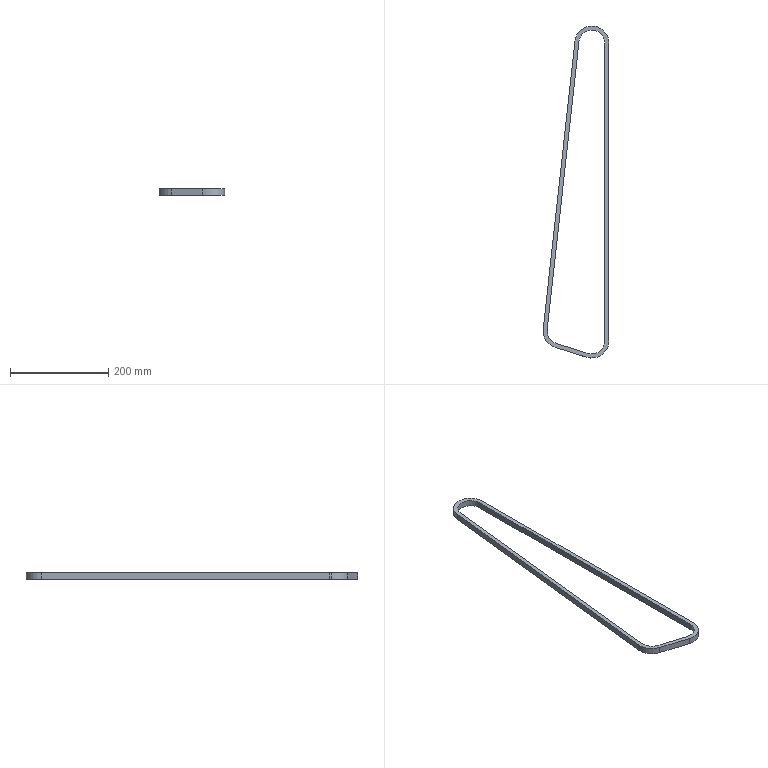Part | STEP file | Belt 1-2^Lifting mechanism | 1 solid | 16 faces | box 133.82 x 674.32 x 12.8 mm | volume 154708 mm3 | cylinder 8 | plane 8 | commonest cylinder face diameters 52.68 x4 69.32 x4
STEP:
#1=CARTESIAN_POINT('',(0.,0.,0.));
#2=DIRECTION('',(0.,0.,1.));
#3=DIRECTION('',(1.,0.,0.));
#4=AXIS2_PLACEMENT_3D('',#1,#2,#3);
#5=CARTESIAN_POINT('',(-90.681,22.887,6.4));
#6=VERTEX_POINT('',#5);
#7=CARTESIAN_POINT('',(-90.681,22.887,-6.4));
#8=VERTEX_POINT('',#7);
#9=CARTESIAN_POINT('',(-90.681,22.887,6.4));
#10=DIRECTION('',(0.,0.,-1.));
#11=VECTOR('',#10,1.);
#12=LINE('',#9,#11);
#13=CARTESIAN_POINT('',(-64.5,20.,6.4));
#14=DIRECTION('',(0.,0.,-1.));
#15=DIRECTION('',(-1.,0.,0.));
#16=AXIS2_PLACEMENT_3D('',#13,#14,#15);
#17=CYLINDRICAL_SURFACE('',#16,26.34);
#18=CARTESIAN_POINT('',(0.1098,0.));
#19=DIRECTION('',(0.,1.));
#20=VECTOR('',#19,1.);
#21=LINE('',#18,#20);
#22=(GEOMETRIC_REPRESENTATION_CONTEXT(2)PARAMETRIC_REPRESENTATION_CONTEXT()REPRESENTATION_CONTEXT('',''));
#23=DEFINITIONAL_REPRESENTATION('',(#21),#22);
#24=PCURVE('',#17,#23);
#25=CARTESIAN_POINT('',(-92.085,10.153,6.4));
#26=DIRECTION('',(0.994,-0.1096,0.));
#27=DIRECTION('',(0.1096,0.994,0.));
#28=AXIS2_PLACEMENT_3D('',#25,#26,#27);
#29=PLANE('',#28);
#30=CARTESIAN_POINT('',(12.811,0.));
#31=DIRECTION('',(0.,-1.));
#32=VECTOR('',#31,1.);
#33=LINE('',#30,#32);
#34=(GEOMETRIC_REPRESENTATION_CONTEXT(2)PARAMETRIC_REPRESENTATION_CONTEXT()REPRESENTATION_CONTEXT('',''));
#35=DEFINITIONAL_REPRESENTATION('',(#33),#34);
#36=PCURVE('',#29,#35);
#37=SURFACE_CURVE('',#12,(#24,#36),.PCURVE_S1.);
#38=EDGE_CURVE('',#6,#8,#37,.T.);
#39=ORIENTED_EDGE('',*,*,#38,.T.);
#40=CARTESIAN_POINT('',(-90.84,20.,-6.4));
#41=VERTEX_POINT('',#40);
#42=CARTESIAN_POINT('',(-64.5,20.,-6.4));
#43=DIRECTION('',(0.,0.,1.));
#44=DIRECTION('',(-1.,0.,0.));
#45=AXIS2_PLACEMENT_3D('',#42,#43,#44);
#46=CIRCLE('',#45,26.34);
#47=CARTESIAN_POINT('',(6.283,12.8));
#48=DIRECTION('',(-1.,0.));
#49=VECTOR('',#48,1.);
#50=LINE('',#47,#49);
#51=(GEOMETRIC_REPRESENTATION_CONTEXT(2)PARAMETRIC_REPRESENTATION_CONTEXT()REPRESENTATION_CONTEXT('',''));
#52=DEFINITIONAL_REPRESENTATION('',(#50),#51);
#53=PCURVE('',#17,#52);
#54=CARTESIAN_POINT('',(0.,0.,-6.4));
#55=DIRECTION('',(0.,0.,-1.));
#56=DIRECTION('',(-1.,0.,0.));
#57=AXIS2_PLACEMENT_3D('',#54,#55,#56);
#58=PLANE('',#57);
#59=CARTESIAN_POINT('',(90.84,20.));
#60=CARTESIAN_POINT('',(90.84,-25.622));
#61=CARTESIAN_POINT('',(51.33,-2.811));
#62=CARTESIAN_POINT('',(11.82,20.));
#63=CARTESIAN_POINT('',(51.33,42.811));
#64=CARTESIAN_POINT('',(90.84,65.622));
#65=CARTESIAN_POINT('',(90.84,20.));
#66=(BOUNDED_CURVE()B_SPLINE_CURVE(2,(#59,#60,#61,#62,#63,#64,#65),.UNSPECIFIED.,.T.,.F.)B_SPLINE_CURVE_WITH_KNOTS((1,2,2,2,2,1),(-2.094,0.,2.094,4.189,6.283,8.378),.UNSPECIFIED.)CURVE()GEOMETRIC_REPRESENTATION_ITEM()RATIONAL_B_SPLINE_CURVE((1.,0.5,1.,0.5,1.,0.5,1.))REPRESENTATION_ITEM(''));
#67=(GEOMETRIC_REPRESENTATION_CONTEXT(2)PARAMETRIC_REPRESENTATION_CONTEXT()REPRESENTATION_CONTEXT('',''));
#68=DEFINITIONAL_REPRESENTATION('',(#66),#67);
#69=PCURVE('',#58,#68);
#70=SURFACE_CURVE('',#46,(#53,#69),.PCURVE_S1.);
#71=EDGE_CURVE('',#8,#41,#70,.T.);
#72=ORIENTED_EDGE('',*,*,#71,.T.);
#73=CARTESIAN_POINT('',(-90.84,20.,6.4));
#74=VERTEX_POINT('',#73);
#75=CARTESIAN_POINT('',(-90.84,20.,6.4));
#76=DIRECTION('',(0.,0.,-1.));
#77=VECTOR('',#76,1.);
#78=LINE('',#75,#77);
#79=CARTESIAN_POINT('',(0.,0.));
#80=DIRECTION('',(0.,1.));
#81=VECTOR('',#80,1.);
#82=LINE('',#79,#81);
#83=(GEOMETRIC_REPRESENTATION_CONTEXT(2)PARAMETRIC_REPRESENTATION_CONTEXT()REPRESENTATION_CONTEXT('',''));
#84=DEFINITIONAL_REPRESENTATION('',(#82),#83);
#85=PCURVE('',#17,#84);
#86=CARTESIAN_POINT('',(-64.5,20.,6.4));
#87=DIRECTION('',(0.,0.,-1.));
#88=DIRECTION('',(-1.,0.,0.));
#89=AXIS2_PLACEMENT_3D('',#86,#87,#88);
#90=CYLINDRICAL_SURFACE('',#89,26.34);
#91=CARTESIAN_POINT('',(6.283,0.));
#92=DIRECTION('',(0.,1.));
#93=VECTOR('',#92,1.);
#94=LINE('',#91,#93);
#95=(GEOMETRIC_REPRESENTATION_CONTEXT(2)PARAMETRIC_REPRESENTATION_CONTEXT()REPRESENTATION_CONTEXT('',''));
#96=DEFINITIONAL_REPRESENTATION('',(#94),#95);
#97=PCURVE('',#90,#96);
#98=SURFACE_CURVE('',#78,(#85,#97),.PCURVE_S1.);
#99=EDGE_CURVE('',#74,#41,#98,.T.);
#100=ORIENTED_EDGE('',*,*,#99,.F.);
#101=CARTESIAN_POINT('',(-64.5,20.,6.4));
#102=DIRECTION('',(0.,0.,1.));
#103=DIRECTION('',(-1.,0.,0.));
#104=AXIS2_PLACEMENT_3D('',#101,#102,#103);
#105=CIRCLE('',#104,26.34);
#106=CARTESIAN_POINT('',(6.283,0.));
#107=DIRECTION('',(-1.,0.));
#108=VECTOR('',#107,1.);
#109=LINE('',#106,#108);
#110=(GEOMETRIC_REPRESENTATION_CONTEXT(2)PARAMETRIC_REPRESENTATION_CONTEXT()REPRESENTATION_CONTEXT('',''));
#111=DEFINITIONAL_REPRESENTATION('',(#109),#110);
#112=PCURVE('',#17,#111);
#113=CARTESIAN_POINT('',(0.,0.,6.4));
#114=DIRECTION('',(0.,0.,-1.));
#115=DIRECTION('',(-1.,0.,0.));
#116=AXIS2_PLACEMENT_3D('',#113,#114,#115);
#117=PLANE('',#116);
#118=CARTESIAN_POINT('',(90.84,20.));
#119=CARTESIAN_POINT('',(90.84,-25.622));
#120=CARTESIAN_POINT('',(51.33,-2.811));
#121=CARTESIAN_POINT('',(11.82,20.));
#122=CARTESIAN_POINT('',(51.33,42.811));
#123=CARTESIAN_POINT('',(90.84,65.622));
#124=CARTESIAN_POINT('',(90.84,20.));
#125=(BOUNDED_CURVE()B_SPLINE_CURVE(2,(#118,#119,#120,#121,#122,#123,#124),.UNSPECIFIED.,.T.,.F.)B_SPLINE_CURVE_WITH_KNOTS((1,2,2,2,2,1),(-2.094,0.,2.094,4.189,6.283,8.378),.UNSPECIFIED.)CURVE()GEOMETRIC_REPRESENTATION_ITEM()RATIONAL_B_SPLINE_CURVE((1.,0.5,1.,0.5,1.,0.5,1.))REPRESENTATION_ITEM(''));
#126=(GEOMETRIC_REPRESENTATION_CONTEXT(2)PARAMETRIC_REPRESENTATION_CONTEXT()REPRESENTATION_CONTEXT('',''));
#127=DEFINITIONAL_REPRESENTATION('',(#125),#126);
#128=PCURVE('',#117,#127);
#129=SURFACE_CURVE('',#105,(#112,#128),.PCURVE_S1.);
#130=EDGE_CURVE('',#6,#74,#129,.T.);
#131=ORIENTED_EDGE('',*,*,#130,.F.);
#132=EDGE_LOOP('',(#39,#72,#100,#131));
#133=FACE_BOUND('',#132,.F.);
#134=ADVANCED_FACE('',(#133),#17,.F.);
#135=CARTESIAN_POINT('',(-99.16,20.,6.4));
#136=VERTEX_POINT('',#135);
#137=CARTESIAN_POINT('',(-74.765,-13.105,6.4));
#138=VERTEX_POINT('',#137);
#139=CARTESIAN_POINT('',(-64.5,20.,6.4));
#140=DIRECTION('',(0.,0.,1.));
#141=DIRECTION('',(-1.,0.,0.));
#142=AXIS2_PLACEMENT_3D('',#139,#140,#141);
#143=CIRCLE('',#142,34.66);
#144=CARTESIAN_POINT('',(-64.5,20.,6.4));
#145=DIRECTION('',(0.,0.,-1.));
#146=DIRECTION('',(-1.,0.,0.));
#147=AXIS2_PLACEMENT_3D('',#144,#145,#146);
#148=CYLINDRICAL_SURFACE('',#147,34.66);
#149=CARTESIAN_POINT('',(6.283,0.));
#150=DIRECTION('',(-1.,0.));
#151=VECTOR('',#150,1.);
#152=LINE('',#149,#151);
#153=(GEOMETRIC_REPRESENTATION_CONTEXT(2)PARAMETRIC_REPRESENTATION_CONTEXT()REPRESENTATION_CONTEXT('',''));
#154=DEFINITIONAL_REPRESENTATION('',(#152),#153);
#155=PCURVE('',#148,#154);
#156=CARTESIAN_POINT('',(99.16,20.));
#157=CARTESIAN_POINT('',(99.16,-40.033));
#158=CARTESIAN_POINT('',(47.17,-10.016));
#159=CARTESIAN_POINT('',(-4.82,20.));
#160=CARTESIAN_POINT('',(47.17,50.016));
#161=CARTESIAN_POINT('',(99.16,80.033));
#162=CARTESIAN_POINT('',(99.16,20.));
#163=(BOUNDED_CURVE()B_SPLINE_CURVE(2,(#156,#157,#158,#159,#160,#161,#162),.UNSPECIFIED.,.T.,.F.)B_SPLINE_CURVE_WITH_KNOTS((1,2,2,2,2,1),(-2.094,0.,2.094,4.189,6.283,8.378),.UNSPECIFIED.)CURVE()GEOMETRIC_REPRESENTATION_ITEM()RATIONAL_B_SPLINE_CURVE((1.,0.5,1.,0.5,1.,0.5,1.))REPRESENTATION_ITEM(''));
#164=(GEOMETRIC_REPRESENTATION_CONTEXT(2)PARAMETRIC_REPRESENTATION_CONTEXT()REPRESENTATION_CONTEXT('',''));
#165=DEFINITIONAL_REPRESENTATION('',(#163),#164);
#166=PCURVE('',#117,#165);
#167=SURFACE_CURVE('',#143,(#155,#166),.PCURVE_S1.);
#168=EDGE_CURVE('',#136,#138,#167,.T.);
#169=ORIENTED_EDGE('',*,*,#168,.F.);
#170=CARTESIAN_POINT('',(-99.16,20.,-6.4));
#171=VERTEX_POINT('',#170);
#172=CARTESIAN_POINT('',(-99.16,20.,6.4));
#173=DIRECTION('',(0.,0.,-1.));
#174=VECTOR('',#173,1.);
#175=LINE('',#172,#174);
#176=CARTESIAN_POINT('',(6.283,0.));
#177=DIRECTION('',(0.,1.));
#178=VECTOR('',#177,1.);
#179=LINE('',#176,#178);
#180=(GEOMETRIC_REPRESENTATION_CONTEXT(2)PARAMETRIC_REPRESENTATION_CONTEXT()REPRESENTATION_CONTEXT('',''));
#181=DEFINITIONAL_REPRESENTATION('',(#179),#180);
#182=PCURVE('',#148,#181);
#183=CARTESIAN_POINT('',(-64.5,20.,6.4));
#184=DIRECTION('',(0.,0.,-1.));
#185=DIRECTION('',(-1.,0.,0.));
#186=AXIS2_PLACEMENT_3D('',#183,#184,#185);
#187=CYLINDRICAL_SURFACE('',#186,34.66);
#188=CARTESIAN_POINT('',(0.,0.));
#189=DIRECTION('',(0.,1.));
#190=VECTOR('',#189,1.);
#191=LINE('',#188,#190);
#192=(GEOMETRIC_REPRESENTATION_CONTEXT(2)PARAMETRIC_REPRESENTATION_CONTEXT()REPRESENTATION_CONTEXT('',''));
#193=DEFINITIONAL_REPRESENTATION('',(#191),#192);
#194=PCURVE('',#187,#193);
#195=SURFACE_CURVE('',#175,(#182,#194),.PCURVE_S1.);
#196=EDGE_CURVE('',#136,#171,#195,.T.);
#197=ORIENTED_EDGE('',*,*,#196,.T.);
#198=CARTESIAN_POINT('',(-74.765,-13.105,-6.4));
#199=VERTEX_POINT('',#198);
#200=CARTESIAN_POINT('',(-64.5,20.,-6.4));
#201=DIRECTION('',(0.,0.,1.));
#202=DIRECTION('',(-1.,0.,0.));
#203=AXIS2_PLACEMENT_3D('',#200,#201,#202);
#204=CIRCLE('',#203,34.66);
#205=CARTESIAN_POINT('',(6.283,12.8));
#206=DIRECTION('',(-1.,0.));
#207=VECTOR('',#206,1.);
#208=LINE('',#205,#207);
#209=(GEOMETRIC_REPRESENTATION_CONTEXT(2)PARAMETRIC_REPRESENTATION_CONTEXT()REPRESENTATION_CONTEXT('',''));
#210=DEFINITIONAL_REPRESENTATION('',(#208),#209);
#211=PCURVE('',#148,#210);
#212=CARTESIAN_POINT('',(99.16,20.));
#213=CARTESIAN_POINT('',(99.16,-40.033));
#214=CARTESIAN_POINT('',(47.17,-10.016));
#215=CARTESIAN_POINT('',(-4.82,20.));
#216=CARTESIAN_POINT('',(47.17,50.016));
#217=CARTESIAN_POINT('',(99.16,80.033));
#218=CARTESIAN_POINT('',(99.16,20.));
#219=(BOUNDED_CURVE()B_SPLINE_CURVE(2,(#212,#213,#214,#215,#216,#217,#218),.UNSPECIFIED.,.T.,.F.)B_SPLINE_CURVE_WITH_KNOTS((1,2,2,2,2,1),(-2.094,0.,2.094,4.189,6.283,8.378),.UNSPECIFIED.)CURVE()GEOMETRIC_REPRESENTATION_ITEM()RATIONAL_B_SPLINE_CURVE((1.,0.5,1.,0.5,1.,0.5,1.))REPRESENTATION_ITEM(''));
#220=(GEOMETRIC_REPRESENTATION_CONTEXT(2)PARAMETRIC_REPRESENTATION_CONTEXT()REPRESENTATION_CONTEXT('',''));
#221=DEFINITIONAL_REPRESENTATION('',(#219),#220);
#222=PCURVE('',#58,#221);
#223=SURFACE_CURVE('',#204,(#211,#222),.PCURVE_S1.);
#224=EDGE_CURVE('',#171,#199,#223,.T.);
#225=ORIENTED_EDGE('',*,*,#224,.T.);
#226=CARTESIAN_POINT('',(-74.765,-13.105,6.4));
#227=DIRECTION('',(0.,0.,-1.));
#228=VECTOR('',#227,1.);
#229=LINE('',#226,#228);
#230=CARTESIAN_POINT('',(5.013,0.));
#231=DIRECTION('',(0.,1.));
#232=VECTOR('',#231,1.);
#233=LINE('',#230,#232);
#234=(GEOMETRIC_REPRESENTATION_CONTEXT(2)PARAMETRIC_REPRESENTATION_CONTEXT()REPRESENTATION_CONTEXT('',''));
#235=DEFINITIONAL_REPRESENTATION('',(#233),#234);
#236=PCURVE('',#148,#235);
#237=CARTESIAN_POINT('',(-10.265,-33.105,6.4));
#238=DIRECTION('',(0.2962,0.9551,0.));
#239=DIRECTION('',(-0.9551,0.2962,0.));
#240=AXIS2_PLACEMENT_3D('',#237,#238,#239);
#241=PLANE('',#240);
#242=CARTESIAN_POINT('',(67.53,0.));
#243=DIRECTION('',(0.,-1.));
#244=VECTOR('',#243,1.);
#245=LINE('',#242,#244);
#246=(GEOMETRIC_REPRESENTATION_CONTEXT(2)PARAMETRIC_REPRESENTATION_CONTEXT()REPRESENTATION_CONTEXT('',''));
#247=DEFINITIONAL_REPRESENTATION('',(#245),#246);
#248=PCURVE('',#241,#247);
#249=SURFACE_CURVE('',#229,(#236,#248),.PCURVE_S1.);
#250=EDGE_CURVE('',#138,#199,#249,.T.);
#251=ORIENTED_EDGE('',*,*,#250,.F.);
#252=EDGE_LOOP('',(#169,#197,#225,#251));
#253=FACE_BOUND('',#252,.T.);
#254=ADVANCED_FACE('',(#253),#148,.T.);
#255=CARTESIAN_POINT('',(-10.265,-33.105,6.4));
#256=VERTEX_POINT('',#255);
#257=CARTESIAN_POINT('',(34.66,0.,6.4));
#258=VERTEX_POINT('',#257);
#259=CARTESIAN_POINT('',(0.,0.,6.4));
#260=DIRECTION('',(0.,0.,1.));
#261=DIRECTION('',(-1.,0.,0.));
#262=AXIS2_PLACEMENT_3D('',#259,#260,#261);
#263=CIRCLE('',#262,34.66);
#264=CARTESIAN_POINT('',(34.66,0.));
#265=CARTESIAN_POINT('',(34.66,-60.033));
#266=CARTESIAN_POINT('',(-17.33,-30.016));
#267=CARTESIAN_POINT('',(-69.32,0.));
#268=CARTESIAN_POINT('',(-17.33,30.016));
#269=CARTESIAN_POINT('',(34.66,60.033));
#270=CARTESIAN_POINT('',(34.66,0.));
#271=(BOUNDED_CURVE()B_SPLINE_CURVE(2,(#264,#265,#266,#267,#268,#269,#270),.UNSPECIFIED.,.T.,.F.)B_SPLINE_CURVE_WITH_KNOTS((1,2,2,2,2,1),(-2.094,0.,2.094,4.189,6.283,8.378),.UNSPECIFIED.)CURVE()GEOMETRIC_REPRESENTATION_ITEM()RATIONAL_B_SPLINE_CURVE((1.,0.5,1.,0.5,1.,0.5,1.))REPRESENTATION_ITEM(''));
#272=(GEOMETRIC_REPRESENTATION_CONTEXT(2)PARAMETRIC_REPRESENTATION_CONTEXT()REPRESENTATION_CONTEXT('',''));
#273=DEFINITIONAL_REPRESENTATION('',(#271),#272);
#274=PCURVE('',#117,#273);
#275=CARTESIAN_POINT('',(0.,0.,6.4));
#276=DIRECTION('',(0.,0.,-1.));
#277=DIRECTION('',(-1.,0.,0.));
#278=AXIS2_PLACEMENT_3D('',#275,#276,#277);
#279=CYLINDRICAL_SURFACE('',#278,34.66);
#280=CARTESIAN_POINT('',(6.283,0.));
#281=DIRECTION('',(-1.,0.));
#282=VECTOR('',#281,1.);
#283=LINE('',#280,#282);
#284=(GEOMETRIC_REPRESENTATION_CONTEXT(2)PARAMETRIC_REPRESENTATION_CONTEXT()REPRESENTATION_CONTEXT('',''));
#285=DEFINITIONAL_REPRESENTATION('',(#283),#284);
#286=PCURVE('',#279,#285);
#287=SURFACE_CURVE('',#263,(#274,#286),.PCURVE_S1.);
#288=EDGE_CURVE('',#256,#258,#287,.T.);
#289=ORIENTED_EDGE('',*,*,#288,.T.);
#290=CARTESIAN_POINT('',(34.66,605.,6.4));
#291=VERTEX_POINT('',#290);
#292=CARTESIAN_POINT('',(34.66,0.,6.4));
#293=DIRECTION('',(0.,1.,0.));
#294=VECTOR('',#293,1.);
#295=LINE('',#292,#294);
#296=CARTESIAN_POINT('',(-34.66,0.));
#297=DIRECTION('',(0.,1.));
#298=VECTOR('',#297,1.);
#299=LINE('',#296,#298);
#300=(GEOMETRIC_REPRESENTATION_CONTEXT(2)PARAMETRIC_REPRESENTATION_CONTEXT()REPRESENTATION_CONTEXT('',''));
#301=DEFINITIONAL_REPRESENTATION('',(#299),#300);
#302=PCURVE('',#117,#301);
#303=CARTESIAN_POINT('',(34.66,0.,6.4));
#304=DIRECTION('',(-1.,0.,0.));
#305=DIRECTION('',(0.,-1.,0.));
#306=AXIS2_PLACEMENT_3D('',#303,#304,#305);
#307=PLANE('',#306);
#308=CARTESIAN_POINT('',(0.,0.));
#309=DIRECTION('',(-1.,0.));
#310=VECTOR('',#309,1.);
#311=LINE('',#308,#310);
#312=(GEOMETRIC_REPRESENTATION_CONTEXT(2)PARAMETRIC_REPRESENTATION_CONTEXT()REPRESENTATION_CONTEXT('',''));
#313=DEFINITIONAL_REPRESENTATION('',(#311),#312);
#314=PCURVE('',#307,#313);
#315=SURFACE_CURVE('',#295,(#302,#314),.PCURVE_S1.);
#316=EDGE_CURVE('',#258,#291,#315,.T.);
#317=ORIENTED_EDGE('',*,*,#316,.T.);
#318=CARTESIAN_POINT('',(-34.451,608.798,6.4));
#319=VERTEX_POINT('',#318);
#320=CARTESIAN_POINT('',(0.,605.,6.4));
#321=DIRECTION('',(0.,0.,1.));
#322=DIRECTION('',(-1.,0.,0.));
#323=AXIS2_PLACEMENT_3D('',#320,#321,#322);
#324=CIRCLE('',#323,34.66);
#325=CARTESIAN_POINT('',(34.66,605.));
#326=CARTESIAN_POINT('',(34.66,544.967));
#327=CARTESIAN_POINT('',(-17.33,574.984));
#328=CARTESIAN_POINT('',(-69.32,605.));
#329=CARTESIAN_POINT('',(-17.33,635.016));
#330=CARTESIAN_POINT('',(34.66,665.033));
#331=CARTESIAN_POINT('',(34.66,605.));
#332=(BOUNDED_CURVE()B_SPLINE_CURVE(2,(#325,#326,#327,#328,#329,#330,#331),.UNSPECIFIED.,.T.,.F.)B_SPLINE_CURVE_WITH_KNOTS((1,2,2,2,2,1),(-2.094,0.,2.094,4.189,6.283,8.378),.UNSPECIFIED.)CURVE()GEOMETRIC_REPRESENTATION_ITEM()RATIONAL_B_SPLINE_CURVE((1.,0.5,1.,0.5,1.,0.5,1.))REPRESENTATION_ITEM(''));
#333=(GEOMETRIC_REPRESENTATION_CONTEXT(2)PARAMETRIC_REPRESENTATION_CONTEXT()REPRESENTATION_CONTEXT('',''));
#334=DEFINITIONAL_REPRESENTATION('',(#332),#333);
#335=PCURVE('',#117,#334);
#336=CARTESIAN_POINT('',(0.,605.,6.4));
#337=DIRECTION('',(0.,0.,-1.));
#338=DIRECTION('',(-1.,0.,0.));
#339=AXIS2_PLACEMENT_3D('',#336,#337,#338);
#340=CYLINDRICAL_SURFACE('',#339,34.66);
#341=CARTESIAN_POINT('',(6.283,0.));
#342=DIRECTION('',(-1.,0.));
#343=VECTOR('',#342,1.);
#344=LINE('',#341,#343);
#345=(GEOMETRIC_REPRESENTATION_CONTEXT(2)PARAMETRIC_REPRESENTATION_CONTEXT()REPRESENTATION_CONTEXT('',''));
#346=DEFINITIONAL_REPRESENTATION('',(#344),#345);
#347=PCURVE('',#340,#346);
#348=SURFACE_CURVE('',#324,(#335,#347),.PCURVE_S1.);
#349=EDGE_CURVE('',#291,#319,#348,.T.);
#350=ORIENTED_EDGE('',*,*,#349,.T.);
#351=CARTESIAN_POINT('',(-98.951,23.798,6.4));
#352=VERTEX_POINT('',#351);
#353=CARTESIAN_POINT('',(-100.355,11.065,6.4));
#354=DIRECTION('',(-0.1096,-0.994,0.));
#355=VECTOR('',#354,1.);
#356=LINE('',#353,#355);
#357=CARTESIAN_POINT('',(100.355,11.065));
#358=DIRECTION('',(0.1096,-0.994));
#359=VECTOR('',#358,1.);
#360=LINE('',#357,#359);
#361=(GEOMETRIC_REPRESENTATION_CONTEXT(2)PARAMETRIC_REPRESENTATION_CONTEXT()REPRESENTATION_CONTEXT('',''));
#362=DEFINITIONAL_REPRESENTATION('',(#360),#361);
#363=PCURVE('',#117,#362);
#364=CARTESIAN_POINT('',(-100.355,11.065,6.4));
#365=DIRECTION('',(0.994,-0.1096,0.));
#366=DIRECTION('',(0.1096,0.994,0.));
#367=AXIS2_PLACEMENT_3D('',#364,#365,#366);
#368=PLANE('',#367);
#369=CARTESIAN_POINT('',(0.,0.));
#370=DIRECTION('',(-1.,0.));
#371=VECTOR('',#370,1.);
#372=LINE('',#369,#371);
#373=(GEOMETRIC_REPRESENTATION_CONTEXT(2)PARAMETRIC_REPRESENTATION_CONTEXT()REPRESENTATION_CONTEXT('',''));
#374=DEFINITIONAL_REPRESENTATION('',(#372),#373);
#375=PCURVE('',#368,#374);
#376=SURFACE_CURVE('',#356,(#363,#375),.PCURVE_S1.);
#377=EDGE_CURVE('',#319,#352,#376,.T.);
#378=ORIENTED_EDGE('',*,*,#377,.T.);
#379=CARTESIAN_POINT('',(-64.5,20.,6.4));
#380=DIRECTION('',(0.,0.,1.));
#381=DIRECTION('',(-1.,0.,0.));
#382=AXIS2_PLACEMENT_3D('',#379,#380,#381);
#383=CIRCLE('',#382,34.66);
#384=CARTESIAN_POINT('',(99.16,20.));
#385=CARTESIAN_POINT('',(99.16,-40.033));
#386=CARTESIAN_POINT('',(47.17,-10.016));
#387=CARTESIAN_POINT('',(-4.82,20.));
#388=CARTESIAN_POINT('',(47.17,50.016));
#389=CARTESIAN_POINT('',(99.16,80.033));
#390=CARTESIAN_POINT('',(99.16,20.));
#391=(BOUNDED_CURVE()B_SPLINE_CURVE(2,(#384,#385,#386,#387,#388,#389,#390),.UNSPECIFIED.,.T.,.F.)B_SPLINE_CURVE_WITH_KNOTS((1,2,2,2,2,1),(-2.094,0.,2.094,4.189,6.283,8.378),.UNSPECIFIED.)CURVE()GEOMETRIC_REPRESENTATION_ITEM()RATIONAL_B_SPLINE_CURVE((1.,0.5,1.,0.5,1.,0.5,1.))REPRESENTATION_ITEM(''));
#392=(GEOMETRIC_REPRESENTATION_CONTEXT(2)PARAMETRIC_REPRESENTATION_CONTEXT()REPRESENTATION_CONTEXT('',''));
#393=DEFINITIONAL_REPRESENTATION('',(#391),#392);
#394=PCURVE('',#117,#393);
#395=CARTESIAN_POINT('',(6.283,0.));
#396=DIRECTION('',(-1.,0.));
#397=VECTOR('',#396,1.);
#398=LINE('',#395,#397);
#399=(GEOMETRIC_REPRESENTATION_CONTEXT(2)PARAMETRIC_REPRESENTATION_CONTEXT()REPRESENTATION_CONTEXT('',''));
#400=DEFINITIONAL_REPRESENTATION('',(#398),#399);
#401=PCURVE('',#187,#400);
#402=SURFACE_CURVE('',#383,(#394,#401),.PCURVE_S1.);
#403=EDGE_CURVE('',#352,#136,#402,.T.);
#404=ORIENTED_EDGE('',*,*,#403,.T.);
#405=ORIENTED_EDGE('',*,*,#168,.T.);
#406=CARTESIAN_POINT('',(-10.265,-33.105,6.4));
#407=DIRECTION('',(0.9551,-0.2962,0.));
#408=VECTOR('',#407,1.);
#409=LINE('',#406,#408);
#410=CARTESIAN_POINT('',(10.265,-33.105));
#411=DIRECTION('',(-0.9551,-0.2962));
#412=VECTOR('',#411,1.);
#413=LINE('',#410,#412);
#414=(GEOMETRIC_REPRESENTATION_CONTEXT(2)PARAMETRIC_REPRESENTATION_CONTEXT()REPRESENTATION_CONTEXT('',''));
#415=DEFINITIONAL_REPRESENTATION('',(#413),#414);
#416=PCURVE('',#117,#415);
#417=CARTESIAN_POINT('',(0.,0.));
#418=DIRECTION('',(-1.,0.));
#419=VECTOR('',#418,1.);
#420=LINE('',#417,#419);
#421=(GEOMETRIC_REPRESENTATION_CONTEXT(2)PARAMETRIC_REPRESENTATION_CONTEXT()REPRESENTATION_CONTEXT('',''));
#422=DEFINITIONAL_REPRESENTATION('',(#420),#421);
#423=PCURVE('',#241,#422);
#424=SURFACE_CURVE('',#409,(#416,#423),.PCURVE_S1.);
#425=EDGE_CURVE('',#138,#256,#424,.T.);
#426=ORIENTED_EDGE('',*,*,#425,.T.);
#427=EDGE_LOOP('',(#289,#317,#350,#378,#404,#405,#426));
#428=FACE_BOUND('',#427,.T.);
#429=CARTESIAN_POINT('',(-7.801,-25.158,6.4));
#430=VERTEX_POINT('',#429);
#431=CARTESIAN_POINT('',(26.34,0.,6.4));
#432=VERTEX_POINT('',#431);
#433=CARTESIAN_POINT('',(0.,0.,6.4));
#434=DIRECTION('',(0.,0.,1.));
#435=DIRECTION('',(-1.,0.,0.));
#436=AXIS2_PLACEMENT_3D('',#433,#434,#435);
#437=CIRCLE('',#436,26.34);
#438=CARTESIAN_POINT('',(26.34,0.));
#439=CARTESIAN_POINT('',(26.34,-45.622));
#440=CARTESIAN_POINT('',(-13.17,-22.811));
#441=CARTESIAN_POINT('',(-52.68,0.));
#442=CARTESIAN_POINT('',(-13.17,22.811));
#443=CARTESIAN_POINT('',(26.34,45.622));
#444=CARTESIAN_POINT('',(26.34,0.));
#445=(BOUNDED_CURVE()B_SPLINE_CURVE(2,(#438,#439,#440,#441,#442,#443,#444),.UNSPECIFIED.,.T.,.F.)B_SPLINE_CURVE_WITH_KNOTS((1,2,2,2,2,1),(-2.094,0.,2.094,4.189,6.283,8.378),.UNSPECIFIED.)CURVE()GEOMETRIC_REPRESENTATION_ITEM()RATIONAL_B_SPLINE_CURVE((1.,0.5,1.,0.5,1.,0.5,1.))REPRESENTATION_ITEM(''));
#446=(GEOMETRIC_REPRESENTATION_CONTEXT(2)PARAMETRIC_REPRESENTATION_CONTEXT()REPRESENTATION_CONTEXT('',''));
#447=DEFINITIONAL_REPRESENTATION('',(#445),#446);
#448=PCURVE('',#117,#447);
#449=CARTESIAN_POINT('',(0.,0.,6.4));
#450=DIRECTION('',(0.,0.,-1.));
#451=DIRECTION('',(-1.,0.,0.));
#452=AXIS2_PLACEMENT_3D('',#449,#450,#451);
#453=CYLINDRICAL_SURFACE('',#452,26.34);
#454=CARTESIAN_POINT('',(6.283,0.));
#455=DIRECTION('',(-1.,0.));
#456=VECTOR('',#455,1.);
#457=LINE('',#454,#456);
#458=(GEOMETRIC_REPRESENTATION_CONTEXT(2)PARAMETRIC_REPRESENTATION_CONTEXT()REPRESENTATION_CONTEXT('',''));
#459=DEFINITIONAL_REPRESENTATION('',(#457),#458);
#460=PCURVE('',#453,#459);
#461=SURFACE_CURVE('',#437,(#448,#460),.PCURVE_S1.);
#462=EDGE_CURVE('',#430,#432,#461,.T.);
#463=ORIENTED_EDGE('',*,*,#462,.F.);
#464=CARTESIAN_POINT('',(-72.301,-5.158,6.4));
#465=VERTEX_POINT('',#464);
#466=CARTESIAN_POINT('',(-7.801,-25.158,6.4));
#467=DIRECTION('',(0.9551,-0.2962,0.));
#468=VECTOR('',#467,1.);
#469=LINE('',#466,#468);
#470=CARTESIAN_POINT('',(7.801,-25.158));
#471=DIRECTION('',(-0.9551,-0.2962));
#472=VECTOR('',#471,1.);
#473=LINE('',#470,#472);
#474=(GEOMETRIC_REPRESENTATION_CONTEXT(2)PARAMETRIC_REPRESENTATION_CONTEXT()REPRESENTATION_CONTEXT('',''));
#475=DEFINITIONAL_REPRESENTATION('',(#473),#474);
#476=PCURVE('',#117,#475);
#477=CARTESIAN_POINT('',(-7.801,-25.158,6.4));
#478=DIRECTION('',(0.2962,0.9551,0.));
#479=DIRECTION('',(-0.9551,0.2962,0.));
#480=AXIS2_PLACEMENT_3D('',#477,#478,#479);
#481=PLANE('',#480);
#482=CARTESIAN_POINT('',(0.,0.));
#483=DIRECTION('',(-1.,0.));
#484=VECTOR('',#483,1.);
#485=LINE('',#482,#484);
#486=(GEOMETRIC_REPRESENTATION_CONTEXT(2)PARAMETRIC_REPRESENTATION_CONTEXT()REPRESENTATION_CONTEXT('',''));
#487=DEFINITIONAL_REPRESENTATION('',(#485),#486);
#488=PCURVE('',#481,#487);
#489=SURFACE_CURVE('',#469,(#476,#488),.PCURVE_S1.);
#490=EDGE_CURVE('',#465,#430,#489,.T.);
#491=ORIENTED_EDGE('',*,*,#490,.F.);
#492=CARTESIAN_POINT('',(-64.5,20.,6.4));
#493=DIRECTION('',(0.,0.,1.));
#494=DIRECTION('',(-1.,0.,0.));
#495=AXIS2_PLACEMENT_3D('',#492,#493,#494);
#496=CIRCLE('',#495,26.34);
#497=CARTESIAN_POINT('',(90.84,20.));
#498=CARTESIAN_POINT('',(90.84,-25.622));
#499=CARTESIAN_POINT('',(51.33,-2.811));
#500=CARTESIAN_POINT('',(11.82,20.));
#501=CARTESIAN_POINT('',(51.33,42.811));
#502=CARTESIAN_POINT('',(90.84,65.622));
#503=CARTESIAN_POINT('',(90.84,20.));
#504=(BOUNDED_CURVE()B_SPLINE_CURVE(2,(#497,#498,#499,#500,#501,#502,#503),.UNSPECIFIED.,.T.,.F.)B_SPLINE_CURVE_WITH_KNOTS((1,2,2,2,2,1),(-2.094,0.,2.094,4.189,6.283,8.378),.UNSPECIFIED.)CURVE()GEOMETRIC_REPRESENTATION_ITEM()RATIONAL_B_SPLINE_CURVE((1.,0.5,1.,0.5,1.,0.5,1.))REPRESENTATION_ITEM(''));
#505=(GEOMETRIC_REPRESENTATION_CONTEXT(2)PARAMETRIC_REPRESENTATION_CONTEXT()REPRESENTATION_CONTEXT('',''));
#506=DEFINITIONAL_REPRESENTATION('',(#504),#505);
#507=PCURVE('',#117,#506);
#508=CARTESIAN_POINT('',(6.283,0.));
#509=DIRECTION('',(-1.,0.));
#510=VECTOR('',#509,1.);
#511=LINE('',#508,#510);
#512=(GEOMETRIC_REPRESENTATION_CONTEXT(2)PARAMETRIC_REPRESENTATION_CONTEXT()REPRESENTATION_CONTEXT('',''));
#513=DEFINITIONAL_REPRESENTATION('',(#511),#512);
#514=PCURVE('',#90,#513);
#515=SURFACE_CURVE('',#496,(#507,#514),.PCURVE_S1.);
#516=EDGE_CURVE('',#74,#465,#515,.T.);
#517=ORIENTED_EDGE('',*,*,#516,.F.);
#518=ORIENTED_EDGE('',*,*,#130,.F.);
#519=CARTESIAN_POINT('',(-26.181,607.887,6.4));
#520=VERTEX_POINT('',#519);
#521=CARTESIAN_POINT('',(-92.085,10.153,6.4));
#522=DIRECTION('',(-0.1096,-0.994,0.));
#523=VECTOR('',#522,1.);
#524=LINE('',#521,#523);
#525=CARTESIAN_POINT('',(92.085,10.153));
#526=DIRECTION('',(0.1096,-0.994));
#527=VECTOR('',#526,1.);
#528=LINE('',#525,#527);
#529=(GEOMETRIC_REPRESENTATION_CONTEXT(2)PARAMETRIC_REPRESENTATION_CONTEXT()REPRESENTATION_CONTEXT('',''));
#530=DEFINITIONAL_REPRESENTATION('',(#528),#529);
#531=PCURVE('',#117,#530);
#532=CARTESIAN_POINT('',(0.,0.));
#533=DIRECTION('',(-1.,0.));
#534=VECTOR('',#533,1.);
#535=LINE('',#532,#534);
#536=(GEOMETRIC_REPRESENTATION_CONTEXT(2)PARAMETRIC_REPRESENTATION_CONTEXT()REPRESENTATION_CONTEXT('',''));
#537=DEFINITIONAL_REPRESENTATION('',(#535),#536);
#538=PCURVE('',#29,#537);
#539=SURFACE_CURVE('',#524,(#531,#538),.PCURVE_S1.);
#540=EDGE_CURVE('',#520,#6,#539,.T.);
#541=ORIENTED_EDGE('',*,*,#540,.F.);
#542=CARTESIAN_POINT('',(26.34,605.,6.4));
#543=VERTEX_POINT('',#542);
#544=CARTESIAN_POINT('',(0.,605.,6.4));
#545=DIRECTION('',(0.,0.,1.));
#546=DIRECTION('',(-1.,0.,0.));
#547=AXIS2_PLACEMENT_3D('',#544,#545,#546);
#548=CIRCLE('',#547,26.34);
#549=CARTESIAN_POINT('',(26.34,605.));
#550=CARTESIAN_POINT('',(26.34,559.378));
#551=CARTESIAN_POINT('',(-13.17,582.189));
#552=CARTESIAN_POINT('',(-52.68,605.));
#553=CARTESIAN_POINT('',(-13.17,627.811));
#554=CARTESIAN_POINT('',(26.34,650.622));
#555=CARTESIAN_POINT('',(26.34,605.));
#556=(BOUNDED_CURVE()B_SPLINE_CURVE(2,(#549,#550,#551,#552,#553,#554,#555),.UNSPECIFIED.,.T.,.F.)B_SPLINE_CURVE_WITH_KNOTS((1,2,2,2,2,1),(-2.094,0.,2.094,4.189,6.283,8.378),.UNSPECIFIED.)CURVE()GEOMETRIC_REPRESENTATION_ITEM()RATIONAL_B_SPLINE_CURVE((1.,0.5,1.,0.5,1.,0.5,1.))REPRESENTATION_ITEM(''));
#557=(GEOMETRIC_REPRESENTATION_CONTEXT(2)PARAMETRIC_REPRESENTATION_CONTEXT()REPRESENTATION_CONTEXT('',''));
#558=DEFINITIONAL_REPRESENTATION('',(#556),#557);
#559=PCURVE('',#117,#558);
#560=CARTESIAN_POINT('',(0.,605.,6.4));
#561=DIRECTION('',(0.,0.,-1.));
#562=DIRECTION('',(-1.,0.,0.));
#563=AXIS2_PLACEMENT_3D('',#560,#561,#562);
#564=CYLINDRICAL_SURFACE('',#563,26.34);
#565=CARTESIAN_POINT('',(6.283,0.));
#566=DIRECTION('',(-1.,0.));
#567=VECTOR('',#566,1.);
#568=LINE('',#565,#567);
#569=(GEOMETRIC_REPRESENTATION_CONTEXT(2)PARAMETRIC_REPRESENTATION_CONTEXT()REPRESENTATION_CONTEXT('',''));
#570=DEFINITIONAL_REPRESENTATION('',(#568),#569);
#571=PCURVE('',#564,#570);
#572=SURFACE_CURVE('',#548,(#559,#571),.PCURVE_S1.);
#573=EDGE_CURVE('',#543,#520,#572,.T.);
#574=ORIENTED_EDGE('',*,*,#573,.F.);
#575=CARTESIAN_POINT('',(26.34,0.,6.4));
#576=DIRECTION('',(0.,1.,0.));
#577=VECTOR('',#576,1.);
#578=LINE('',#575,#577);
#579=CARTESIAN_POINT('',(-26.34,0.));
#580=DIRECTION('',(0.,1.));
#581=VECTOR('',#580,1.);
#582=LINE('',#579,#581);
#583=(GEOMETRIC_REPRESENTATION_CONTEXT(2)PARAMETRIC_REPRESENTATION_CONTEXT()REPRESENTATION_CONTEXT('',''));
#584=DEFINITIONAL_REPRESENTATION('',(#582),#583);
#585=PCURVE('',#117,#584);
#586=CARTESIAN_POINT('',(26.34,0.,6.4));
#587=DIRECTION('',(-1.,0.,0.));
#588=DIRECTION('',(0.,-1.,0.));
#589=AXIS2_PLACEMENT_3D('',#586,#587,#588);
#590=PLANE('',#589);
#591=CARTESIAN_POINT('',(0.,0.));
#592=DIRECTION('',(-1.,0.));
#593=VECTOR('',#592,1.);
#594=LINE('',#591,#593);
#595=(GEOMETRIC_REPRESENTATION_CONTEXT(2)PARAMETRIC_REPRESENTATION_CONTEXT()REPRESENTATION_CONTEXT('',''));
#596=DEFINITIONAL_REPRESENTATION('',(#594),#595);
#597=PCURVE('',#590,#596);
#598=SURFACE_CURVE('',#578,(#585,#597),.PCURVE_S1.);
#599=EDGE_CURVE('',#432,#543,#598,.T.);
#600=ORIENTED_EDGE('',*,*,#599,.F.);
#601=EDGE_LOOP('',(#463,#491,#517,#518,#541,#574,#600));
#602=FACE_BOUND('',#601,.T.);
#603=ADVANCED_FACE('',(#428,#602),#117,.F.);
#604=CARTESIAN_POINT('',(-10.265,-33.105,-6.4));
#605=VERTEX_POINT('',#604);
#606=CARTESIAN_POINT('',(34.66,0.,-6.4));
#607=VERTEX_POINT('',#606);
#608=CARTESIAN_POINT('',(0.,0.,-6.4));
#609=DIRECTION('',(0.,0.,1.));
#610=DIRECTION('',(-1.,0.,0.));
#611=AXIS2_PLACEMENT_3D('',#608,#609,#610);
#612=CIRCLE('',#611,34.66);
#613=CARTESIAN_POINT('',(34.66,0.));
#614=CARTESIAN_POINT('',(34.66,-60.033));
#615=CARTESIAN_POINT('',(-17.33,-30.016));
#616=CARTESIAN_POINT('',(-69.32,0.));
#617=CARTESIAN_POINT('',(-17.33,30.016));
#618=CARTESIAN_POINT('',(34.66,60.033));
#619=CARTESIAN_POINT('',(34.66,0.));
#620=(BOUNDED_CURVE()B_SPLINE_CURVE(2,(#613,#614,#615,#616,#617,#618,#619),.UNSPECIFIED.,.T.,.F.)B_SPLINE_CURVE_WITH_KNOTS((1,2,2,2,2,1),(-2.094,0.,2.094,4.189,6.283,8.378),.UNSPECIFIED.)CURVE()GEOMETRIC_REPRESENTATION_ITEM()RATIONAL_B_SPLINE_CURVE((1.,0.5,1.,0.5,1.,0.5,1.))REPRESENTATION_ITEM(''));
#621=(GEOMETRIC_REPRESENTATION_CONTEXT(2)PARAMETRIC_REPRESENTATION_CONTEXT()REPRESENTATION_CONTEXT('',''));
#622=DEFINITIONAL_REPRESENTATION('',(#620),#621);
#623=PCURVE('',#58,#622);
#624=CARTESIAN_POINT('',(6.283,12.8));
#625=DIRECTION('',(-1.,0.));
#626=VECTOR('',#625,1.);
#627=LINE('',#624,#626);
#628=(GEOMETRIC_REPRESENTATION_CONTEXT(2)PARAMETRIC_REPRESENTATION_CONTEXT()REPRESENTATION_CONTEXT('',''));
#629=DEFINITIONAL_REPRESENTATION('',(#627),#628);
#630=PCURVE('',#279,#629);
#631=SURFACE_CURVE('',#612,(#623,#630),.PCURVE_S1.);
#632=EDGE_CURVE('',#605,#607,#631,.T.);
#633=ORIENTED_EDGE('',*,*,#632,.F.);
#634=CARTESIAN_POINT('',(-10.265,-33.105,-6.4));
#635=DIRECTION('',(0.9551,-0.2962,0.));
#636=VECTOR('',#635,1.);
#637=LINE('',#634,#636);
#638=CARTESIAN_POINT('',(10.265,-33.105));
#639=DIRECTION('',(-0.9551,-0.2962));
#640=VECTOR('',#639,1.);
#641=LINE('',#638,#640);
#642=(GEOMETRIC_REPRESENTATION_CONTEXT(2)PARAMETRIC_REPRESENTATION_CONTEXT()REPRESENTATION_CONTEXT('',''));
#643=DEFINITIONAL_REPRESENTATION('',(#641),#642);
#644=PCURVE('',#58,#643);
#645=CARTESIAN_POINT('',(0.,-12.8));
#646=DIRECTION('',(-1.,0.));
#647=VECTOR('',#646,1.);
#648=LINE('',#645,#647);
#649=(GEOMETRIC_REPRESENTATION_CONTEXT(2)PARAMETRIC_REPRESENTATION_CONTEXT()REPRESENTATION_CONTEXT('',''));
#650=DEFINITIONAL_REPRESENTATION('',(#648),#649);
#651=PCURVE('',#241,#650);
#652=SURFACE_CURVE('',#637,(#644,#651),.PCURVE_S1.);
#653=EDGE_CURVE('',#199,#605,#652,.T.);
#654=ORIENTED_EDGE('',*,*,#653,.F.);
#655=ORIENTED_EDGE('',*,*,#224,.F.);
#656=CARTESIAN_POINT('',(-98.951,23.798,-6.4));
#657=VERTEX_POINT('',#656);
#658=CARTESIAN_POINT('',(-64.5,20.,-6.4));
#659=DIRECTION('',(0.,0.,1.));
#660=DIRECTION('',(-1.,0.,0.));
#661=AXIS2_PLACEMENT_3D('',#658,#659,#660);
#662=CIRCLE('',#661,34.66);
#663=CARTESIAN_POINT('',(99.16,20.));
#664=CARTESIAN_POINT('',(99.16,-40.033));
#665=CARTESIAN_POINT('',(47.17,-10.016));
#666=CARTESIAN_POINT('',(-4.82,20.));
#667=CARTESIAN_POINT('',(47.17,50.016));
#668=CARTESIAN_POINT('',(99.16,80.033));
#669=CARTESIAN_POINT('',(99.16,20.));
#670=(BOUNDED_CURVE()B_SPLINE_CURVE(2,(#663,#664,#665,#666,#667,#668,#669),.UNSPECIFIED.,.T.,.F.)B_SPLINE_CURVE_WITH_KNOTS((1,2,2,2,2,1),(-2.094,0.,2.094,4.189,6.283,8.378),.UNSPECIFIED.)CURVE()GEOMETRIC_REPRESENTATION_ITEM()RATIONAL_B_SPLINE_CURVE((1.,0.5,1.,0.5,1.,0.5,1.))REPRESENTATION_ITEM(''));
#671=(GEOMETRIC_REPRESENTATION_CONTEXT(2)PARAMETRIC_REPRESENTATION_CONTEXT()REPRESENTATION_CONTEXT('',''));
#672=DEFINITIONAL_REPRESENTATION('',(#670),#671);
#673=PCURVE('',#58,#672);
#674=CARTESIAN_POINT('',(6.283,12.8));
#675=DIRECTION('',(-1.,0.));
#676=VECTOR('',#675,1.);
#677=LINE('',#674,#676);
#678=(GEOMETRIC_REPRESENTATION_CONTEXT(2)PARAMETRIC_REPRESENTATION_CONTEXT()REPRESENTATION_CONTEXT('',''));
#679=DEFINITIONAL_REPRESENTATION('',(#677),#678);
#680=PCURVE('',#187,#679);
#681=SURFACE_CURVE('',#662,(#673,#680),.PCURVE_S1.);
#682=EDGE_CURVE('',#657,#171,#681,.T.);
#683=ORIENTED_EDGE('',*,*,#682,.F.);
#684=CARTESIAN_POINT('',(-34.451,608.798,-6.4));
#685=VERTEX_POINT('',#684);
#686=CARTESIAN_POINT('',(-100.355,11.065,-6.4));
#687=DIRECTION('',(-0.1096,-0.994,0.));
#688=VECTOR('',#687,1.);
#689=LINE('',#686,#688);
#690=CARTESIAN_POINT('',(100.355,11.065));
#691=DIRECTION('',(0.1096,-0.994));
#692=VECTOR('',#691,1.);
#693=LINE('',#690,#692);
#694=(GEOMETRIC_REPRESENTATION_CONTEXT(2)PARAMETRIC_REPRESENTATION_CONTEXT()REPRESENTATION_CONTEXT('',''));
#695=DEFINITIONAL_REPRESENTATION('',(#693),#694);
#696=PCURVE('',#58,#695);
#697=CARTESIAN_POINT('',(0.,-12.8));
#698=DIRECTION('',(-1.,0.));
#699=VECTOR('',#698,1.);
#700=LINE('',#697,#699);
#701=(GEOMETRIC_REPRESENTATION_CONTEXT(2)PARAMETRIC_REPRESENTATION_CONTEXT()REPRESENTATION_CONTEXT('',''));
#702=DEFINITIONAL_REPRESENTATION('',(#700),#701);
#703=PCURVE('',#368,#702);
#704=SURFACE_CURVE('',#689,(#696,#703),.PCURVE_S1.);
#705=EDGE_CURVE('',#685,#657,#704,.T.);
#706=ORIENTED_EDGE('',*,*,#705,.F.);
#707=CARTESIAN_POINT('',(34.66,605.,-6.4));
#708=VERTEX_POINT('',#707);
#709=CARTESIAN_POINT('',(0.,605.,-6.4));
#710=DIRECTION('',(0.,0.,1.));
#711=DIRECTION('',(-1.,0.,0.));
#712=AXIS2_PLACEMENT_3D('',#709,#710,#711);
#713=CIRCLE('',#712,34.66);
#714=CARTESIAN_POINT('',(34.66,605.));
#715=CARTESIAN_POINT('',(34.66,544.967));
#716=CARTESIAN_POINT('',(-17.33,574.984));
#717=CARTESIAN_POINT('',(-69.32,605.));
#718=CARTESIAN_POINT('',(-17.33,635.016));
#719=CARTESIAN_POINT('',(34.66,665.033));
#720=CARTESIAN_POINT('',(34.66,605.));
#721=(BOUNDED_CURVE()B_SPLINE_CURVE(2,(#714,#715,#716,#717,#718,#719,#720),.UNSPECIFIED.,.T.,.F.)B_SPLINE_CURVE_WITH_KNOTS((1,2,2,2,2,1),(-2.094,0.,2.094,4.189,6.283,8.378),.UNSPECIFIED.)CURVE()GEOMETRIC_REPRESENTATION_ITEM()RATIONAL_B_SPLINE_CURVE((1.,0.5,1.,0.5,1.,0.5,1.))REPRESENTATION_ITEM(''));
#722=(GEOMETRIC_REPRESENTATION_CONTEXT(2)PARAMETRIC_REPRESENTATION_CONTEXT()REPRESENTATION_CONTEXT('',''));
#723=DEFINITIONAL_REPRESENTATION('',(#721),#722);
#724=PCURVE('',#58,#723);
#725=CARTESIAN_POINT('',(6.283,12.8));
#726=DIRECTION('',(-1.,0.));
#727=VECTOR('',#726,1.);
#728=LINE('',#725,#727);
#729=(GEOMETRIC_REPRESENTATION_CONTEXT(2)PARAMETRIC_REPRESENTATION_CONTEXT()REPRESENTATION_CONTEXT('',''));
#730=DEFINITIONAL_REPRESENTATION('',(#728),#729);
#731=PCURVE('',#340,#730);
#732=SURFACE_CURVE('',#713,(#724,#731),.PCURVE_S1.);
#733=EDGE_CURVE('',#708,#685,#732,.T.);
#734=ORIENTED_EDGE('',*,*,#733,.F.);
#735=CARTESIAN_POINT('',(34.66,0.,-6.4));
#736=DIRECTION('',(0.,1.,0.));
#737=VECTOR('',#736,1.);
#738=LINE('',#735,#737);
#739=CARTESIAN_POINT('',(-34.66,0.));
#740=DIRECTION('',(0.,1.));
#741=VECTOR('',#740,1.);
#742=LINE('',#739,#741);
#743=(GEOMETRIC_REPRESENTATION_CONTEXT(2)PARAMETRIC_REPRESENTATION_CONTEXT()REPRESENTATION_CONTEXT('',''));
#744=DEFINITIONAL_REPRESENTATION('',(#742),#743);
#745=PCURVE('',#58,#744);
#746=CARTESIAN_POINT('',(0.,-12.8));
#747=DIRECTION('',(-1.,0.));
#748=VECTOR('',#747,1.);
#749=LINE('',#746,#748);
#750=(GEOMETRIC_REPRESENTATION_CONTEXT(2)PARAMETRIC_REPRESENTATION_CONTEXT()REPRESENTATION_CONTEXT('',''));
#751=DEFINITIONAL_REPRESENTATION('',(#749),#750);
#752=PCURVE('',#307,#751);
#753=SURFACE_CURVE('',#738,(#745,#752),.PCURVE_S1.);
#754=EDGE_CURVE('',#607,#708,#753,.T.);
#755=ORIENTED_EDGE('',*,*,#754,.F.);
#756=EDGE_LOOP('',(#633,#654,#655,#683,#706,#734,#755));
#757=FACE_BOUND('',#756,.T.);
#758=CARTESIAN_POINT('',(-72.301,-5.158,-6.4));
#759=VERTEX_POINT('',#758);
#760=CARTESIAN_POINT('',(-7.801,-25.158,-6.4));
#761=VERTEX_POINT('',#760);
#762=CARTESIAN_POINT('',(-7.801,-25.158,-6.4));
#763=DIRECTION('',(0.9551,-0.2962,0.));
#764=VECTOR('',#763,1.);
#765=LINE('',#762,#764);
#766=CARTESIAN_POINT('',(7.801,-25.158));
#767=DIRECTION('',(-0.9551,-0.2962));
#768=VECTOR('',#767,1.);
#769=LINE('',#766,#768);
#770=(GEOMETRIC_REPRESENTATION_CONTEXT(2)PARAMETRIC_REPRESENTATION_CONTEXT()REPRESENTATION_CONTEXT('',''));
#771=DEFINITIONAL_REPRESENTATION('',(#769),#770);
#772=PCURVE('',#58,#771);
#773=CARTESIAN_POINT('',(0.,-12.8));
#774=DIRECTION('',(-1.,0.));
#775=VECTOR('',#774,1.);
#776=LINE('',#773,#775);
#777=(GEOMETRIC_REPRESENTATION_CONTEXT(2)PARAMETRIC_REPRESENTATION_CONTEXT()REPRESENTATION_CONTEXT('',''));
#778=DEFINITIONAL_REPRESENTATION('',(#776),#777);
#779=PCURVE('',#481,#778);
#780=SURFACE_CURVE('',#765,(#772,#779),.PCURVE_S1.);
#781=EDGE_CURVE('',#759,#761,#780,.T.);
#782=ORIENTED_EDGE('',*,*,#781,.T.);
#783=CARTESIAN_POINT('',(26.34,0.,-6.4));
#784=VERTEX_POINT('',#783);
#785=CARTESIAN_POINT('',(0.,0.,-6.4));
#786=DIRECTION('',(0.,0.,1.));
#787=DIRECTION('',(-1.,0.,0.));
#788=AXIS2_PLACEMENT_3D('',#785,#786,#787);
#789=CIRCLE('',#788,26.34);
#790=CARTESIAN_POINT('',(26.34,0.));
#791=CARTESIAN_POINT('',(26.34,-45.622));
#792=CARTESIAN_POINT('',(-13.17,-22.811));
#793=CARTESIAN_POINT('',(-52.68,0.));
#794=CARTESIAN_POINT('',(-13.17,22.811));
#795=CARTESIAN_POINT('',(26.34,45.622));
#796=CARTESIAN_POINT('',(26.34,0.));
#797=(BOUNDED_CURVE()B_SPLINE_CURVE(2,(#790,#791,#792,#793,#794,#795,#796),.UNSPECIFIED.,.T.,.F.)B_SPLINE_CURVE_WITH_KNOTS((1,2,2,2,2,1),(-2.094,0.,2.094,4.189,6.283,8.378),.UNSPECIFIED.)CURVE()GEOMETRIC_REPRESENTATION_ITEM()RATIONAL_B_SPLINE_CURVE((1.,0.5,1.,0.5,1.,0.5,1.))REPRESENTATION_ITEM(''));
#798=(GEOMETRIC_REPRESENTATION_CONTEXT(2)PARAMETRIC_REPRESENTATION_CONTEXT()REPRESENTATION_CONTEXT('',''));
#799=DEFINITIONAL_REPRESENTATION('',(#797),#798);
#800=PCURVE('',#58,#799);
#801=CARTESIAN_POINT('',(6.283,12.8));
#802=DIRECTION('',(-1.,0.));
#803=VECTOR('',#802,1.);
#804=LINE('',#801,#803);
#805=(GEOMETRIC_REPRESENTATION_CONTEXT(2)PARAMETRIC_REPRESENTATION_CONTEXT()REPRESENTATION_CONTEXT('',''));
#806=DEFINITIONAL_REPRESENTATION('',(#804),#805);
#807=PCURVE('',#453,#806);
#808=SURFACE_CURVE('',#789,(#800,#807),.PCURVE_S1.);
#809=EDGE_CURVE('',#761,#784,#808,.T.);
#810=ORIENTED_EDGE('',*,*,#809,.T.);
#811=CARTESIAN_POINT('',(26.34,605.,-6.4));
#812=VERTEX_POINT('',#811);
#813=CARTESIAN_POINT('',(26.34,0.,-6.4));
#814=DIRECTION('',(0.,1.,0.));
#815=VECTOR('',#814,1.);
#816=LINE('',#813,#815);
#817=CARTESIAN_POINT('',(-26.34,0.));
#818=DIRECTION('',(0.,1.));
#819=VECTOR('',#818,1.);
#820=LINE('',#817,#819);
#821=(GEOMETRIC_REPRESENTATION_CONTEXT(2)PARAMETRIC_REPRESENTATION_CONTEXT()REPRESENTATION_CONTEXT('',''));
#822=DEFINITIONAL_REPRESENTATION('',(#820),#821);
#823=PCURVE('',#58,#822);
#824=CARTESIAN_POINT('',(0.,-12.8));
#825=DIRECTION('',(-1.,0.));
#826=VECTOR('',#825,1.);
#827=LINE('',#824,#826);
#828=(GEOMETRIC_REPRESENTATION_CONTEXT(2)PARAMETRIC_REPRESENTATION_CONTEXT()REPRESENTATION_CONTEXT('',''));
#829=DEFINITIONAL_REPRESENTATION('',(#827),#828);
#830=PCURVE('',#590,#829);
#831=SURFACE_CURVE('',#816,(#823,#830),.PCURVE_S1.);
#832=EDGE_CURVE('',#784,#812,#831,.T.);
#833=ORIENTED_EDGE('',*,*,#832,.T.);
#834=CARTESIAN_POINT('',(-26.181,607.887,-6.4));
#835=VERTEX_POINT('',#834);
#836=CARTESIAN_POINT('',(0.,605.,-6.4));
#837=DIRECTION('',(0.,0.,1.));
#838=DIRECTION('',(-1.,0.,0.));
#839=AXIS2_PLACEMENT_3D('',#836,#837,#838);
#840=CIRCLE('',#839,26.34);
#841=CARTESIAN_POINT('',(26.34,605.));
#842=CARTESIAN_POINT('',(26.34,559.378));
#843=CARTESIAN_POINT('',(-13.17,582.189));
#844=CARTESIAN_POINT('',(-52.68,605.));
#845=CARTESIAN_POINT('',(-13.17,627.811));
#846=CARTESIAN_POINT('',(26.34,650.622));
#847=CARTESIAN_POINT('',(26.34,605.));
#848=(BOUNDED_CURVE()B_SPLINE_CURVE(2,(#841,#842,#843,#844,#845,#846,#847),.UNSPECIFIED.,.T.,.F.)B_SPLINE_CURVE_WITH_KNOTS((1,2,2,2,2,1),(-2.094,0.,2.094,4.189,6.283,8.378),.UNSPECIFIED.)CURVE()GEOMETRIC_REPRESENTATION_ITEM()RATIONAL_B_SPLINE_CURVE((1.,0.5,1.,0.5,1.,0.5,1.))REPRESENTATION_ITEM(''));
#849=(GEOMETRIC_REPRESENTATION_CONTEXT(2)PARAMETRIC_REPRESENTATION_CONTEXT()REPRESENTATION_CONTEXT('',''));
#850=DEFINITIONAL_REPRESENTATION('',(#848),#849);
#851=PCURVE('',#58,#850);
#852=CARTESIAN_POINT('',(6.283,12.8));
#853=DIRECTION('',(-1.,0.));
#854=VECTOR('',#853,1.);
#855=LINE('',#852,#854);
#856=(GEOMETRIC_REPRESENTATION_CONTEXT(2)PARAMETRIC_REPRESENTATION_CONTEXT()REPRESENTATION_CONTEXT('',''));
#857=DEFINITIONAL_REPRESENTATION('',(#855),#856);
#858=PCURVE('',#564,#857);
#859=SURFACE_CURVE('',#840,(#851,#858),.PCURVE_S1.);
#860=EDGE_CURVE('',#812,#835,#859,.T.);
#861=ORIENTED_EDGE('',*,*,#860,.T.);
#862=CARTESIAN_POINT('',(-92.085,10.153,-6.4));
#863=DIRECTION('',(-0.1096,-0.994,0.));
#864=VECTOR('',#863,1.);
#865=LINE('',#862,#864);
#866=CARTESIAN_POINT('',(92.085,10.153));
#867=DIRECTION('',(0.1096,-0.994));
#868=VECTOR('',#867,1.);
#869=LINE('',#866,#868);
#870=(GEOMETRIC_REPRESENTATION_CONTEXT(2)PARAMETRIC_REPRESENTATION_CONTEXT()REPRESENTATION_CONTEXT('',''));
#871=DEFINITIONAL_REPRESENTATION('',(#869),#870);
#872=PCURVE('',#58,#871);
#873=CARTESIAN_POINT('',(0.,-12.8));
#874=DIRECTION('',(-1.,0.));
#875=VECTOR('',#874,1.);
#876=LINE('',#873,#875);
#877=(GEOMETRIC_REPRESENTATION_CONTEXT(2)PARAMETRIC_REPRESENTATION_CONTEXT()REPRESENTATION_CONTEXT('',''));
#878=DEFINITIONAL_REPRESENTATION('',(#876),#877);
#879=PCURVE('',#29,#878);
#880=SURFACE_CURVE('',#865,(#872,#879),.PCURVE_S1.);
#881=EDGE_CURVE('',#835,#8,#880,.T.);
#882=ORIENTED_EDGE('',*,*,#881,.T.);
#883=ORIENTED_EDGE('',*,*,#71,.T.);
#884=CARTESIAN_POINT('',(-64.5,20.,-6.4));
#885=DIRECTION('',(0.,0.,1.));
#886=DIRECTION('',(-1.,0.,0.));
#887=AXIS2_PLACEMENT_3D('',#884,#885,#886);
#888=CIRCLE('',#887,26.34);
#889=CARTESIAN_POINT('',(90.84,20.));
#890=CARTESIAN_POINT('',(90.84,-25.622));
#891=CARTESIAN_POINT('',(51.33,-2.811));
#892=CARTESIAN_POINT('',(11.82,20.));
#893=CARTESIAN_POINT('',(51.33,42.811));
#894=CARTESIAN_POINT('',(90.84,65.622));
#895=CARTESIAN_POINT('',(90.84,20.));
#896=(BOUNDED_CURVE()B_SPLINE_CURVE(2,(#889,#890,#891,#892,#893,#894,#895),.UNSPECIFIED.,.T.,.F.)B_SPLINE_CURVE_WITH_KNOTS((1,2,2,2,2,1),(-2.094,0.,2.094,4.189,6.283,8.378),.UNSPECIFIED.)CURVE()GEOMETRIC_REPRESENTATION_ITEM()RATIONAL_B_SPLINE_CURVE((1.,0.5,1.,0.5,1.,0.5,1.))REPRESENTATION_ITEM(''));
#897=(GEOMETRIC_REPRESENTATION_CONTEXT(2)PARAMETRIC_REPRESENTATION_CONTEXT()REPRESENTATION_CONTEXT('',''));
#898=DEFINITIONAL_REPRESENTATION('',(#896),#897);
#899=PCURVE('',#58,#898);
#900=CARTESIAN_POINT('',(6.283,12.8));
#901=DIRECTION('',(-1.,0.));
#902=VECTOR('',#901,1.);
#903=LINE('',#900,#902);
#904=(GEOMETRIC_REPRESENTATION_CONTEXT(2)PARAMETRIC_REPRESENTATION_CONTEXT()REPRESENTATION_CONTEXT('',''));
#905=DEFINITIONAL_REPRESENTATION('',(#903),#904);
#906=PCURVE('',#90,#905);
#907=SURFACE_CURVE('',#888,(#899,#906),.PCURVE_S1.);
#908=EDGE_CURVE('',#41,#759,#907,.T.);
#909=ORIENTED_EDGE('',*,*,#908,.T.);
#910=EDGE_LOOP('',(#782,#810,#833,#861,#882,#883,#909));
#911=FACE_BOUND('',#910,.T.);
#912=ADVANCED_FACE('',(#757,#911),#58,.T.);
#913=ORIENTED_EDGE('',*,*,#632,.T.);
#914=CARTESIAN_POINT('',(34.66,0.,6.4));
#915=DIRECTION('',(0.,0.,-1.));
#916=VECTOR('',#915,1.);
#917=LINE('',#914,#916);
#918=CARTESIAN_POINT('',(3.142,0.));
#919=DIRECTION('',(0.,1.));
#920=VECTOR('',#919,1.);
#921=LINE('',#918,#920);
#922=(GEOMETRIC_REPRESENTATION_CONTEXT(2)PARAMETRIC_REPRESENTATION_CONTEXT()REPRESENTATION_CONTEXT('',''));
#923=DEFINITIONAL_REPRESENTATION('',(#921),#922);
#924=PCURVE('',#279,#923);
#925=CARTESIAN_POINT('',(0.,0.));
#926=DIRECTION('',(0.,-1.));
#927=VECTOR('',#926,1.);
#928=LINE('',#925,#927);
#929=(GEOMETRIC_REPRESENTATION_CONTEXT(2)PARAMETRIC_REPRESENTATION_CONTEXT()REPRESENTATION_CONTEXT('',''));
#930=DEFINITIONAL_REPRESENTATION('',(#928),#929);
#931=PCURVE('',#307,#930);
#932=SURFACE_CURVE('',#917,(#924,#931),.PCURVE_S1.);
#933=EDGE_CURVE('',#258,#607,#932,.T.);
#934=ORIENTED_EDGE('',*,*,#933,.F.);
#935=ORIENTED_EDGE('',*,*,#288,.F.);
#936=CARTESIAN_POINT('',(-10.265,-33.105,6.4));
#937=DIRECTION('',(0.,0.,-1.));
#938=VECTOR('',#937,1.);
#939=LINE('',#936,#938);
#940=CARTESIAN_POINT('',(5.013,0.));
#941=DIRECTION('',(0.,1.));
#942=VECTOR('',#941,1.);
#943=LINE('',#940,#942);
#944=(GEOMETRIC_REPRESENTATION_CONTEXT(2)PARAMETRIC_REPRESENTATION_CONTEXT()REPRESENTATION_CONTEXT('',''));
#945=DEFINITIONAL_REPRESENTATION('',(#943),#944);
#946=PCURVE('',#279,#945);
#947=CARTESIAN_POINT('',(0.,0.));
#948=DIRECTION('',(0.,-1.));
#949=VECTOR('',#948,1.);
#950=LINE('',#947,#949);
#951=(GEOMETRIC_REPRESENTATION_CONTEXT(2)PARAMETRIC_REPRESENTATION_CONTEXT()REPRESENTATION_CONTEXT('',''));
#952=DEFINITIONAL_REPRESENTATION('',(#950),#951);
#953=PCURVE('',#241,#952);
#954=SURFACE_CURVE('',#939,(#946,#953),.PCURVE_S1.);
#955=EDGE_CURVE('',#256,#605,#954,.T.);
#956=ORIENTED_EDGE('',*,*,#955,.T.);
#957=EDGE_LOOP('',(#913,#934,#935,#956));
#958=FACE_BOUND('',#957,.T.);
#959=ADVANCED_FACE('',(#958),#279,.T.);
#960=ORIENTED_EDGE('',*,*,#754,.T.);
#961=CARTESIAN_POINT('',(34.66,605.,6.4));
#962=DIRECTION('',(0.,0.,-1.));
#963=VECTOR('',#962,1.);
#964=LINE('',#961,#963);
#965=CARTESIAN_POINT('',(-605.,0.));
#966=DIRECTION('',(0.,-1.));
#967=VECTOR('',#966,1.);
#968=LINE('',#965,#967);
#969=(GEOMETRIC_REPRESENTATION_CONTEXT(2)PARAMETRIC_REPRESENTATION_CONTEXT()REPRESENTATION_CONTEXT('',''));
#970=DEFINITIONAL_REPRESENTATION('',(#968),#969);
#971=PCURVE('',#307,#970);
#972=CARTESIAN_POINT('',(3.142,0.));
#973=DIRECTION('',(0.,1.));
#974=VECTOR('',#973,1.);
#975=LINE('',#972,#974);
#976=(GEOMETRIC_REPRESENTATION_CONTEXT(2)PARAMETRIC_REPRESENTATION_CONTEXT()REPRESENTATION_CONTEXT('',''));
#977=DEFINITIONAL_REPRESENTATION('',(#975),#976);
#978=PCURVE('',#340,#977);
#979=SURFACE_CURVE('',#964,(#971,#978),.PCURVE_S1.);
#980=EDGE_CURVE('',#291,#708,#979,.T.);
#981=ORIENTED_EDGE('',*,*,#980,.F.);
#982=ORIENTED_EDGE('',*,*,#316,.F.);
#983=ORIENTED_EDGE('',*,*,#933,.T.);
#984=EDGE_LOOP('',(#960,#981,#982,#983));
#985=FACE_BOUND('',#984,.T.);
#986=ADVANCED_FACE('',(#985),#307,.F.);
#987=ORIENTED_EDGE('',*,*,#733,.T.);
#988=CARTESIAN_POINT('',(-34.451,608.798,6.4));
#989=DIRECTION('',(0.,0.,-1.));
#990=VECTOR('',#989,1.);
#991=LINE('',#988,#990);
#992=CARTESIAN_POINT('',(0.1098,0.));
#993=DIRECTION('',(0.,1.));
#994=VECTOR('',#993,1.);
#995=LINE('',#992,#994);
#996=(GEOMETRIC_REPRESENTATION_CONTEXT(2)PARAMETRIC_REPRESENTATION_CONTEXT()REPRESENTATION_CONTEXT('',''));
#997=DEFINITIONAL_REPRESENTATION('',(#995),#996);
#998=PCURVE('',#340,#997);
#999=CARTESIAN_POINT('',(601.356,0.));
#1000=DIRECTION('',(0.,-1.));
#1001=VECTOR('',#1000,1.);
#1002=LINE('',#999,#1001);
#1003=(GEOMETRIC_REPRESENTATION_CONTEXT(2)PARAMETRIC_REPRESENTATION_CONTEXT()REPRESENTATION_CONTEXT('',''));
#1004=DEFINITIONAL_REPRESENTATION('',(#1002),#1003);
#1005=PCURVE('',#368,#1004);
#1006=SURFACE_CURVE('',#991,(#998,#1005),.PCURVE_S1.);
#1007=EDGE_CURVE('',#319,#685,#1006,.T.);
#1008=ORIENTED_EDGE('',*,*,#1007,.F.);
#1009=ORIENTED_EDGE('',*,*,#349,.F.);
#1010=ORIENTED_EDGE('',*,*,#980,.T.);
#1011=EDGE_LOOP('',(#987,#1008,#1009,#1010));
#1012=FACE_BOUND('',#1011,.T.);
#1013=ADVANCED_FACE('',(#1012),#340,.T.);
#1014=ORIENTED_EDGE('',*,*,#705,.T.);
#1015=CARTESIAN_POINT('',(-98.951,23.798,6.4));
#1016=DIRECTION('',(0.,0.,-1.));
#1017=VECTOR('',#1016,1.);
#1018=LINE('',#1015,#1017);
#1019=CARTESIAN_POINT('',(12.811,0.));
#1020=DIRECTION('',(0.,-1.));
#1021=VECTOR('',#1020,1.);
#1022=LINE('',#1019,#1021);
#1023=(GEOMETRIC_REPRESENTATION_CONTEXT(2)PARAMETRIC_REPRESENTATION_CONTEXT()REPRESENTATION_CONTEXT('',''));
#1024=DEFINITIONAL_REPRESENTATION('',(#1022),#1023);
#1025=PCURVE('',#368,#1024);
#1026=CARTESIAN_POINT('',(0.1098,0.));
#1027=DIRECTION('',(0.,1.));
#1028=VECTOR('',#1027,1.);
#1029=LINE('',#1026,#1028);
#1030=(GEOMETRIC_REPRESENTATION_CONTEXT(2)PARAMETRIC_REPRESENTATION_CONTEXT()REPRESENTATION_CONTEXT('',''));
#1031=DEFINITIONAL_REPRESENTATION('',(#1029),#1030);
#1032=PCURVE('',#187,#1031);
#1033=SURFACE_CURVE('',#1018,(#1025,#1032),.PCURVE_S1.);
#1034=EDGE_CURVE('',#352,#657,#1033,.T.);
#1035=ORIENTED_EDGE('',*,*,#1034,.F.);
#1036=ORIENTED_EDGE('',*,*,#377,.F.);
#1037=ORIENTED_EDGE('',*,*,#1007,.T.);
#1038=EDGE_LOOP('',(#1014,#1035,#1036,#1037));
#1039=FACE_BOUND('',#1038,.T.);
#1040=ADVANCED_FACE('',(#1039),#368,.F.);
#1041=ORIENTED_EDGE('',*,*,#196,.F.);
#1042=ORIENTED_EDGE('',*,*,#403,.F.);
#1043=ORIENTED_EDGE('',*,*,#1034,.T.);
#1044=ORIENTED_EDGE('',*,*,#682,.T.);
#1045=EDGE_LOOP('',(#1041,#1042,#1043,#1044));
#1046=FACE_BOUND('',#1045,.T.);
#1047=ADVANCED_FACE('',(#1046),#187,.T.);
#1048=ORIENTED_EDGE('',*,*,#653,.T.);
#1049=ORIENTED_EDGE('',*,*,#955,.F.);
#1050=ORIENTED_EDGE('',*,*,#425,.F.);
#1051=ORIENTED_EDGE('',*,*,#250,.T.);
#1052=EDGE_LOOP('',(#1048,#1049,#1050,#1051));
#1053=FACE_BOUND('',#1052,.T.);
#1054=ADVANCED_FACE('',(#1053),#241,.F.);
#1055=CARTESIAN_POINT('',(26.34,0.,6.4));
#1056=DIRECTION('',(0.,0.,-1.));
#1057=VECTOR('',#1056,1.);
#1058=LINE('',#1055,#1057);
#1059=CARTESIAN_POINT('',(3.142,0.));
#1060=DIRECTION('',(0.,1.));
#1061=VECTOR('',#1060,1.);
#1062=LINE('',#1059,#1061);
#1063=(GEOMETRIC_REPRESENTATION_CONTEXT(2)PARAMETRIC_REPRESENTATION_CONTEXT()REPRESENTATION_CONTEXT('',''));
#1064=DEFINITIONAL_REPRESENTATION('',(#1062),#1063);
#1065=PCURVE('',#453,#1064);
#1066=CARTESIAN_POINT('',(0.,0.));
#1067=DIRECTION('',(0.,-1.));
#1068=VECTOR('',#1067,1.);
#1069=LINE('',#1066,#1068);
#1070=(GEOMETRIC_REPRESENTATION_CONTEXT(2)PARAMETRIC_REPRESENTATION_CONTEXT()REPRESENTATION_CONTEXT('',''));
#1071=DEFINITIONAL_REPRESENTATION('',(#1069),#1070);
#1072=PCURVE('',#590,#1071);
#1073=SURFACE_CURVE('',#1058,(#1065,#1072),.PCURVE_S1.);
#1074=EDGE_CURVE('',#432,#784,#1073,.T.);
#1075=ORIENTED_EDGE('',*,*,#1074,.F.);
#1076=ORIENTED_EDGE('',*,*,#462,.F.);
#1077=CARTESIAN_POINT('',(-7.801,-25.158,6.4));
#1078=DIRECTION('',(0.,0.,-1.));
#1079=VECTOR('',#1078,1.);
#1080=LINE('',#1077,#1079);
#1081=CARTESIAN_POINT('',(5.013,0.));
#1082=DIRECTION('',(0.,1.));
#1083=VECTOR('',#1082,1.);
#1084=LINE('',#1081,#1083);
#1085=(GEOMETRIC_REPRESENTATION_CONTEXT(2)PARAMETRIC_REPRESENTATION_CONTEXT()REPRESENTATION_CONTEXT('',''));
#1086=DEFINITIONAL_REPRESENTATION('',(#1084),#1085);
#1087=PCURVE('',#453,#1086);
#1088=CARTESIAN_POINT('',(0.,0.));
#1089=DIRECTION('',(0.,-1.));
#1090=VECTOR('',#1089,1.);
#1091=LINE('',#1088,#1090);
#1092=(GEOMETRIC_REPRESENTATION_CONTEXT(2)PARAMETRIC_REPRESENTATION_CONTEXT()REPRESENTATION_CONTEXT('',''));
#1093=DEFINITIONAL_REPRESENTATION('',(#1091),#1092);
#1094=PCURVE('',#481,#1093);
#1095=SURFACE_CURVE('',#1080,(#1087,#1094),.PCURVE_S1.);
#1096=EDGE_CURVE('',#430,#761,#1095,.T.);
#1097=ORIENTED_EDGE('',*,*,#1096,.T.);
#1098=ORIENTED_EDGE('',*,*,#809,.T.);
#1099=EDGE_LOOP('',(#1075,#1076,#1097,#1098));
#1100=FACE_BOUND('',#1099,.F.);
#1101=ADVANCED_FACE('',(#1100),#453,.F.);
#1102=ORIENTED_EDGE('',*,*,#832,.F.);
#1103=ORIENTED_EDGE('',*,*,#1074,.F.);
#1104=ORIENTED_EDGE('',*,*,#599,.T.);
#1105=CARTESIAN_POINT('',(26.34,605.,6.4));
#1106=DIRECTION('',(0.,0.,-1.));
#1107=VECTOR('',#1106,1.);
#1108=LINE('',#1105,#1107);
#1109=CARTESIAN_POINT('',(-605.,0.));
#1110=DIRECTION('',(0.,-1.));
#1111=VECTOR('',#1110,1.);
#1112=LINE('',#1109,#1111);
#1113=(GEOMETRIC_REPRESENTATION_CONTEXT(2)PARAMETRIC_REPRESENTATION_CONTEXT()REPRESENTATION_CONTEXT('',''));
#1114=DEFINITIONAL_REPRESENTATION('',(#1112),#1113);
#1115=PCURVE('',#590,#1114);
#1116=CARTESIAN_POINT('',(3.142,0.));
#1117=DIRECTION('',(0.,1.));
#1118=VECTOR('',#1117,1.);
#1119=LINE('',#1116,#1118);
#1120=(GEOMETRIC_REPRESENTATION_CONTEXT(2)PARAMETRIC_REPRESENTATION_CONTEXT()REPRESENTATION_CONTEXT('',''));
#1121=DEFINITIONAL_REPRESENTATION('',(#1119),#1120);
#1122=PCURVE('',#564,#1121);
#1123=SURFACE_CURVE('',#1108,(#1115,#1122),.PCURVE_S1.);
#1124=EDGE_CURVE('',#543,#812,#1123,.T.);
#1125=ORIENTED_EDGE('',*,*,#1124,.T.);
#1126=EDGE_LOOP('',(#1102,#1103,#1104,#1125));
#1127=FACE_BOUND('',#1126,.T.);
#1128=ADVANCED_FACE('',(#1127),#590,.T.);
#1129=CARTESIAN_POINT('',(-26.181,607.887,6.4));
#1130=DIRECTION('',(0.,0.,-1.));
#1131=VECTOR('',#1130,1.);
#1132=LINE('',#1129,#1131);
#1133=CARTESIAN_POINT('',(0.1098,0.));
#1134=DIRECTION('',(0.,1.));
#1135=VECTOR('',#1134,1.);
#1136=LINE('',#1133,#1135);
#1137=(GEOMETRIC_REPRESENTATION_CONTEXT(2)PARAMETRIC_REPRESENTATION_CONTEXT()REPRESENTATION_CONTEXT('',''));
#1138=DEFINITIONAL_REPRESENTATION('',(#1136),#1137);
#1139=PCURVE('',#564,#1138);
#1140=CARTESIAN_POINT('',(601.356,0.));
#1141=DIRECTION('',(0.,-1.));
#1142=VECTOR('',#1141,1.);
#1143=LINE('',#1140,#1142);
#1144=(GEOMETRIC_REPRESENTATION_CONTEXT(2)PARAMETRIC_REPRESENTATION_CONTEXT()REPRESENTATION_CONTEXT('',''));
#1145=DEFINITIONAL_REPRESENTATION('',(#1143),#1144);
#1146=PCURVE('',#29,#1145);
#1147=SURFACE_CURVE('',#1132,(#1139,#1146),.PCURVE_S1.);
#1148=EDGE_CURVE('',#520,#835,#1147,.T.);
#1149=ORIENTED_EDGE('',*,*,#1148,.F.);
#1150=ORIENTED_EDGE('',*,*,#573,.F.);
#1151=ORIENTED_EDGE('',*,*,#1124,.T.);
#1152=ORIENTED_EDGE('',*,*,#860,.T.);
#1153=EDGE_LOOP('',(#1149,#1150,#1151,#1152));
#1154=FACE_BOUND('',#1153,.F.);
#1155=ADVANCED_FACE('',(#1154),#564,.F.);
#1156=ORIENTED_EDGE('',*,*,#881,.F.);
#1157=ORIENTED_EDGE('',*,*,#1148,.F.);
#1158=ORIENTED_EDGE('',*,*,#540,.T.);
#1159=ORIENTED_EDGE('',*,*,#38,.T.);
#1160=EDGE_LOOP('',(#1156,#1157,#1158,#1159));
#1161=FACE_BOUND('',#1160,.T.);
#1162=ADVANCED_FACE('',(#1161),#29,.T.);
#1163=ORIENTED_EDGE('',*,*,#908,.T.);
#1164=CARTESIAN_POINT('',(-72.301,-5.158,6.4));
#1165=DIRECTION('',(0.,0.,-1.));
#1166=VECTOR('',#1165,1.);
#1167=LINE('',#1164,#1166);
#1168=CARTESIAN_POINT('',(5.013,0.));
#1169=DIRECTION('',(0.,1.));
#1170=VECTOR('',#1169,1.);
#1171=LINE('',#1168,#1170);
#1172=(GEOMETRIC_REPRESENTATION_CONTEXT(2)PARAMETRIC_REPRESENTATION_CONTEXT()REPRESENTATION_CONTEXT('',''));
#1173=DEFINITIONAL_REPRESENTATION('',(#1171),#1172);
#1174=PCURVE('',#90,#1173);
#1175=CARTESIAN_POINT('',(67.53,0.));
#1176=DIRECTION('',(0.,-1.));
#1177=VECTOR('',#1176,1.);
#1178=LINE('',#1175,#1177);
#1179=(GEOMETRIC_REPRESENTATION_CONTEXT(2)PARAMETRIC_REPRESENTATION_CONTEXT()REPRESENTATION_CONTEXT('',''));
#1180=DEFINITIONAL_REPRESENTATION('',(#1178),#1179);
#1181=PCURVE('',#481,#1180);
#1182=SURFACE_CURVE('',#1167,(#1174,#1181),.PCURVE_S1.);
#1183=EDGE_CURVE('',#465,#759,#1182,.T.);
#1184=ORIENTED_EDGE('',*,*,#1183,.F.);
#1185=ORIENTED_EDGE('',*,*,#516,.F.);
#1186=ORIENTED_EDGE('',*,*,#99,.T.);
#1187=EDGE_LOOP('',(#1163,#1184,#1185,#1186));
#1188=FACE_BOUND('',#1187,.F.);
#1189=ADVANCED_FACE('',(#1188),#90,.F.);
#1190=ORIENTED_EDGE('',*,*,#781,.F.);
#1191=ORIENTED_EDGE('',*,*,#1183,.F.);
#1192=ORIENTED_EDGE('',*,*,#490,.T.);
#1193=ORIENTED_EDGE('',*,*,#1096,.T.);
#1194=EDGE_LOOP('',(#1190,#1191,#1192,#1193));
#1195=FACE_BOUND('',#1194,.T.);
#1196=ADVANCED_FACE('',(#1195),#481,.T.);
#1197=CLOSED_SHELL('',(#134,#254,#603,#912,#959,#986,#1013,#1040,#1047,#1054,#1101,#1128,#1155,#1162,#1189,#1196));
#1198=MANIFOLD_SOLID_BREP('',#1197);
#1199=(LENGTH_UNIT()NAMED_UNIT(*)SI_UNIT(.MILLI.,.METRE.));
#1200=UNCERTAINTY_MEASURE_WITH_UNIT(LENGTH_MEASURE(0.0000001),#1199,'','');
#1201=(NAMED_UNIT(*)PLANE_ANGLE_UNIT()SI_UNIT($,.RADIAN.));
#1202=(NAMED_UNIT(*)SI_UNIT($,.STERADIAN.)SOLID_ANGLE_UNIT());
#1203=(GEOMETRIC_REPRESENTATION_CONTEXT(3)GLOBAL_UNCERTAINTY_ASSIGNED_CONTEXT((#1200))GLOBAL_UNIT_ASSIGNED_CONTEXT((#1199,#1201,#1202))REPRESENTATION_CONTEXT('',''));
#1204=ADVANCED_BREP_SHAPE_REPRESENTATION('',(#4,#1198),#1203);